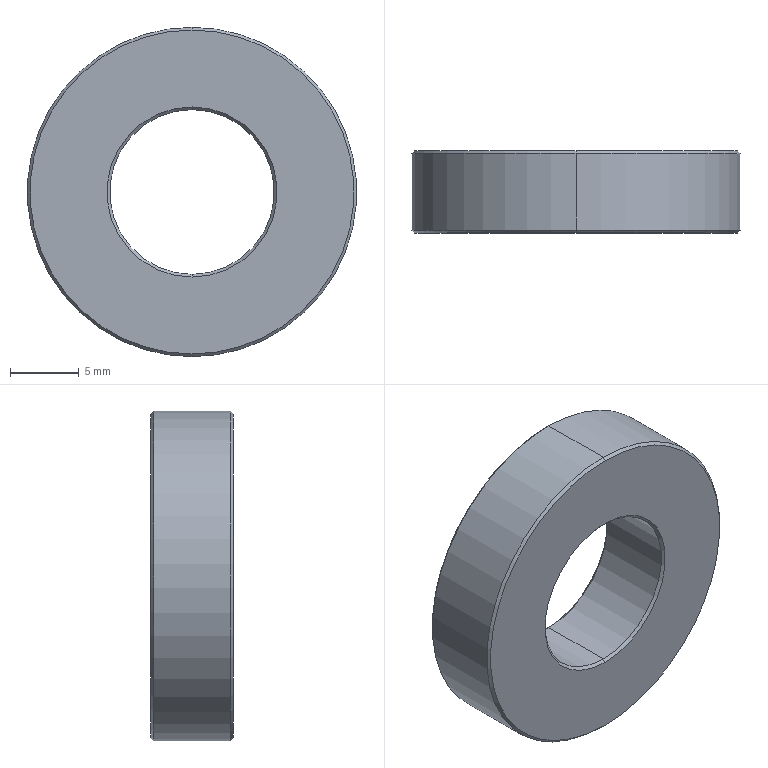Part | SolidWorks | features Chamfer 1, Extrusion 1 | 1 solid | 14 faces | box 24 x 6 x 24 mm | volume 2031 mm3 | cone 8 | cylinder 4 | plane 2 | commonest cylinder face diameters 12 x2 24 x2
STEP:
#1=CARTESIAN_POINT('',(0.,5.8,-6.));
#2=VERTEX_POINT('',#1);
#3=CARTESIAN_POINT('',(0.,5.8,6.));
#4=VERTEX_POINT('',#3);
#5=CARTESIAN_POINT('',(0.,5.8,0.));
#6=DIRECTION('',(0.,1.,0.));
#7=DIRECTION('',(0.,0.,1.));
#8=AXIS2_PLACEMENT_3D('',#5,#6,#7);
#9=CIRCLE('',#8,6.);
#10=EDGE_CURVE('',#2,#4,#9,.T.);
#11=ORIENTED_EDGE('',*,*,#10,.F.);
#12=CARTESIAN_POINT('',(0.,6.,-6.2));
#13=VERTEX_POINT('',#12);
#14=CARTESIAN_POINT('',(0.,5.8,-6.));
#15=DIRECTION('',(0.,0.7071,-0.7071));
#16=VECTOR('',#15,1000.);
#17=LINE('',#14,#16);
#18=EDGE_CURVE('',#2,#13,#17,.T.);
#19=ORIENTED_EDGE('',*,*,#18,.T.);
#20=CARTESIAN_POINT('',(0.,6.,6.2));
#21=VERTEX_POINT('',#20);
#22=CARTESIAN_POINT('',(0.,6.,0.));
#23=DIRECTION('',(0.,-1.,0.));
#24=DIRECTION('',(0.,0.,1.));
#25=AXIS2_PLACEMENT_3D('',#22,#23,#24);
#26=CIRCLE('',#25,6.2);
#27=EDGE_CURVE('',#21,#13,#26,.T.);
#28=ORIENTED_EDGE('',*,*,#27,.F.);
#29=CARTESIAN_POINT('',(0.,5.8,6.));
#30=DIRECTION('',(0.,0.7071,0.7071));
#31=VECTOR('',#30,1000.);
#32=LINE('',#29,#31);
#33=EDGE_CURVE('',#4,#21,#32,.T.);
#34=ORIENTED_EDGE('',*,*,#33,.F.);
#35=EDGE_LOOP('',(#11,#19,#28,#34));
#36=FACE_OUTER_BOUND('',#35,.T.);
#37=CARTESIAN_POINT('',(0.,5.8,0.));
#38=DIRECTION('',(0.,1.,0.));
#39=DIRECTION('',(0.,0.,1.));
#40=AXIS2_PLACEMENT_3D('',#37,#38,#39);
#41=CONICAL_SURFACE('',#40,6.,0.7854);
#42=ADVANCED_FACE('',(#36),#41,.F.);
#43=CARTESIAN_POINT('',(0.,6.,11.8));
#44=VERTEX_POINT('',#43);
#45=CARTESIAN_POINT('',(0.,6.,-11.8));
#46=VERTEX_POINT('',#45);
#47=CARTESIAN_POINT('',(0.,6.,0.));
#48=DIRECTION('',(0.,1.,0.));
#49=DIRECTION('',(0.,0.,1.));
#50=AXIS2_PLACEMENT_3D('',#47,#48,#49);
#51=CIRCLE('',#50,11.8);
#52=EDGE_CURVE('',#44,#46,#51,.T.);
#53=ORIENTED_EDGE('',*,*,#52,.F.);
#54=CARTESIAN_POINT('',(0.,5.8,12.));
#55=VERTEX_POINT('',#54);
#56=CARTESIAN_POINT('',(0.,6.,11.8));
#57=DIRECTION('',(0.,-0.7071,0.7071));
#58=VECTOR('',#57,1000.);
#59=LINE('',#56,#58);
#60=EDGE_CURVE('',#44,#55,#59,.T.);
#61=ORIENTED_EDGE('',*,*,#60,.T.);
#62=CARTESIAN_POINT('',(0.,5.8,-12.));
#63=VERTEX_POINT('',#62);
#64=CARTESIAN_POINT('',(0.,5.8,0.));
#65=DIRECTION('',(0.,-1.,0.));
#66=DIRECTION('',(0.,0.,1.));
#67=AXIS2_PLACEMENT_3D('',#64,#65,#66);
#68=CIRCLE('',#67,12.);
#69=EDGE_CURVE('',#63,#55,#68,.T.);
#70=ORIENTED_EDGE('',*,*,#69,.F.);
#71=CARTESIAN_POINT('',(0.,6.,-11.8));
#72=DIRECTION('',(0.,-0.7071,-0.7071));
#73=VECTOR('',#72,1000.);
#74=LINE('',#71,#73);
#75=EDGE_CURVE('',#46,#63,#74,.T.);
#76=ORIENTED_EDGE('',*,*,#75,.F.);
#77=EDGE_LOOP('',(#53,#61,#70,#76));
#78=FACE_OUTER_BOUND('',#77,.T.);
#79=CARTESIAN_POINT('',(0.,6.,0.));
#80=DIRECTION('',(0.,-1.,0.));
#81=DIRECTION('',(0.,0.,-1.));
#82=AXIS2_PLACEMENT_3D('',#79,#80,#81);
#83=CONICAL_SURFACE('',#82,11.8,0.7854);
#84=ADVANCED_FACE('',(#78),#83,.T.);
#85=CARTESIAN_POINT('',(0.,0.2,6.));
#86=VERTEX_POINT('',#85);
#87=CARTESIAN_POINT('',(0.,0.2,-6.));
#88=VERTEX_POINT('',#87);
#89=CARTESIAN_POINT('',(0.,0.2,0.));
#90=DIRECTION('',(0.,-1.,0.));
#91=DIRECTION('',(0.,0.,1.));
#92=AXIS2_PLACEMENT_3D('',#89,#90,#91);
#93=CIRCLE('',#92,6.);
#94=EDGE_CURVE('',#86,#88,#93,.T.);
#95=ORIENTED_EDGE('',*,*,#94,.F.);
#96=CARTESIAN_POINT('',(0.,0.,6.2));
#97=VERTEX_POINT('',#96);
#98=CARTESIAN_POINT('',(0.,0.,6.2));
#99=DIRECTION('',(0.,-0.7071,0.7071));
#100=VECTOR('',#99,1000.);
#101=LINE('',#98,#100);
#102=EDGE_CURVE('',#86,#97,#101,.T.);
#103=ORIENTED_EDGE('',*,*,#102,.T.);
#104=CARTESIAN_POINT('',(0.,0.,-6.2));
#105=VERTEX_POINT('',#104);
#106=CARTESIAN_POINT('',(0.,0.,0.));
#107=DIRECTION('',(0.,1.,0.));
#108=DIRECTION('',(0.,0.,1.));
#109=AXIS2_PLACEMENT_3D('',#106,#107,#108);
#110=CIRCLE('',#109,6.2);
#111=EDGE_CURVE('',#105,#97,#110,.T.);
#112=ORIENTED_EDGE('',*,*,#111,.F.);
#113=CARTESIAN_POINT('',(0.,0.,-6.2));
#114=DIRECTION('',(0.,-0.7071,-0.7071));
#115=VECTOR('',#114,1000.);
#116=LINE('',#113,#115);
#117=EDGE_CURVE('',#88,#105,#116,.T.);
#118=ORIENTED_EDGE('',*,*,#117,.F.);
#119=EDGE_LOOP('',(#95,#103,#112,#118));
#120=FACE_OUTER_BOUND('',#119,.T.);
#121=CARTESIAN_POINT('',(0.,0.,0.));
#122=DIRECTION('',(0.,-1.,0.));
#123=DIRECTION('',(0.,0.,-1.));
#124=AXIS2_PLACEMENT_3D('',#121,#122,#123);
#125=CONICAL_SURFACE('',#124,6.2,0.7854);
#126=ADVANCED_FACE('',(#120),#125,.F.);
#127=CARTESIAN_POINT('',(0.,0.,-11.8));
#128=VERTEX_POINT('',#127);
#129=CARTESIAN_POINT('',(0.,0.,11.8));
#130=VERTEX_POINT('',#129);
#131=CARTESIAN_POINT('',(0.,0.,0.));
#132=DIRECTION('',(0.,-1.,0.));
#133=DIRECTION('',(0.,0.,1.));
#134=AXIS2_PLACEMENT_3D('',#131,#132,#133);
#135=CIRCLE('',#134,11.8);
#136=EDGE_CURVE('',#128,#130,#135,.T.);
#137=ORIENTED_EDGE('',*,*,#136,.F.);
#138=CARTESIAN_POINT('',(0.,0.2,-12.));
#139=VERTEX_POINT('',#138);
#140=CARTESIAN_POINT('',(0.,0.2,-12.));
#141=DIRECTION('',(0.,0.7071,-0.7071));
#142=VECTOR('',#141,1000.);
#143=LINE('',#140,#142);
#144=EDGE_CURVE('',#128,#139,#143,.T.);
#145=ORIENTED_EDGE('',*,*,#144,.T.);
#146=CARTESIAN_POINT('',(0.,0.2,12.));
#147=VERTEX_POINT('',#146);
#148=CARTESIAN_POINT('',(0.,0.2,0.));
#149=DIRECTION('',(0.,1.,0.));
#150=DIRECTION('',(0.,0.,1.));
#151=AXIS2_PLACEMENT_3D('',#148,#149,#150);
#152=CIRCLE('',#151,12.);
#153=EDGE_CURVE('',#147,#139,#152,.T.);
#154=ORIENTED_EDGE('',*,*,#153,.F.);
#155=CARTESIAN_POINT('',(0.,0.2,12.));
#156=DIRECTION('',(0.,0.7071,0.7071));
#157=VECTOR('',#156,1000.);
#158=LINE('',#155,#157);
#159=EDGE_CURVE('',#130,#147,#158,.T.);
#160=ORIENTED_EDGE('',*,*,#159,.F.);
#161=EDGE_LOOP('',(#137,#145,#154,#160));
#162=FACE_OUTER_BOUND('',#161,.T.);
#163=CARTESIAN_POINT('',(0.,0.2,0.));
#164=DIRECTION('',(0.,1.,0.));
#165=DIRECTION('',(0.,0.,1.));
#166=AXIS2_PLACEMENT_3D('',#163,#164,#165);
#167=CONICAL_SURFACE('',#166,12.,0.7854);
#168=ADVANCED_FACE('',(#162),#167,.T.);
#169=ORIENTED_EDGE('',*,*,#10,.T.);
#170=CARTESIAN_POINT('',(0.,6.,6.));
#171=DIRECTION('',(0.,-1.,0.));
#172=VECTOR('',#171,1000.);
#173=LINE('',#170,#172);
#174=EDGE_CURVE('',#4,#86,#173,.T.);
#175=ORIENTED_EDGE('',*,*,#174,.T.);
#176=ORIENTED_EDGE('',*,*,#94,.T.);
#177=CARTESIAN_POINT('',(0.,6.,-6.));
#178=DIRECTION('',(0.,-1.,0.));
#179=VECTOR('',#178,1000.);
#180=LINE('',#177,#179);
#181=EDGE_CURVE('',#2,#88,#180,.T.);
#182=ORIENTED_EDGE('',*,*,#181,.F.);
#183=EDGE_LOOP('',(#169,#175,#176,#182));
#184=FACE_OUTER_BOUND('',#183,.T.);
#185=CARTESIAN_POINT('',(0.,6.,0.));
#186=DIRECTION('',(0.,-1.,0.));
#187=DIRECTION('',(0.,0.,-1.));
#188=AXIS2_PLACEMENT_3D('',#185,#186,#187);
#189=CYLINDRICAL_SURFACE('',#188,6.);
#190=ADVANCED_FACE('',(#184),#189,.F.);
#191=ORIENTED_EDGE('',*,*,#69,.T.);
#192=CARTESIAN_POINT('',(0.,6.,12.));
#193=DIRECTION('',(0.,-1.,0.));
#194=VECTOR('',#193,1000.);
#195=LINE('',#192,#194);
#196=EDGE_CURVE('',#55,#147,#195,.T.);
#197=ORIENTED_EDGE('',*,*,#196,.T.);
#198=ORIENTED_EDGE('',*,*,#153,.T.);
#199=CARTESIAN_POINT('',(0.,6.,-12.));
#200=DIRECTION('',(0.,-1.,0.));
#201=VECTOR('',#200,1000.);
#202=LINE('',#199,#201);
#203=EDGE_CURVE('',#63,#139,#202,.T.);
#204=ORIENTED_EDGE('',*,*,#203,.F.);
#205=EDGE_LOOP('',(#191,#197,#198,#204));
#206=FACE_OUTER_BOUND('',#205,.T.);
#207=CARTESIAN_POINT('',(0.,6.,0.));
#208=DIRECTION('',(0.,-1.,0.));
#209=DIRECTION('',(0.,0.,-1.));
#210=AXIS2_PLACEMENT_3D('',#207,#208,#209);
#211=CYLINDRICAL_SURFACE('',#210,12.);
#212=ADVANCED_FACE('',(#206),#211,.T.);
#213=CARTESIAN_POINT('',(0.,6.,0.));
#214=DIRECTION('',(0.,1.,0.));
#215=DIRECTION('',(0.,0.,1.));
#216=AXIS2_PLACEMENT_3D('',#213,#214,#215);
#217=CIRCLE('',#216,11.8);
#218=EDGE_CURVE('',#46,#44,#217,.T.);
#219=ORIENTED_EDGE('',*,*,#218,.T.);
#220=ORIENTED_EDGE('',*,*,#52,.T.);
#221=EDGE_LOOP('',(#219,#220));
#222=FACE_OUTER_BOUND('',#221,.T.);
#223=ORIENTED_EDGE('',*,*,#27,.T.);
#224=CARTESIAN_POINT('',(0.,6.,0.));
#225=DIRECTION('',(0.,-1.,0.));
#226=DIRECTION('',(0.,0.,1.));
#227=AXIS2_PLACEMENT_3D('',#224,#225,#226);
#228=CIRCLE('',#227,6.2);
#229=EDGE_CURVE('',#13,#21,#228,.T.);
#230=ORIENTED_EDGE('',*,*,#229,.T.);
#231=EDGE_LOOP('',(#223,#230));
#232=FACE_BOUND('',#231,.T.);
#233=CARTESIAN_POINT('',(0.,6.,0.));
#234=DIRECTION('',(0.,1.,0.));
#235=DIRECTION('',(0.,0.,1.));
#236=AXIS2_PLACEMENT_3D('',#233,#234,#235);
#237=PLANE('',#236);
#238=ADVANCED_FACE('',(#222,#232),#237,.T.);
#239=CARTESIAN_POINT('',(0.,0.,0.));
#240=DIRECTION('',(0.,-1.,0.));
#241=DIRECTION('',(0.,0.,1.));
#242=AXIS2_PLACEMENT_3D('',#239,#240,#241);
#243=CIRCLE('',#242,11.8);
#244=EDGE_CURVE('',#130,#128,#243,.T.);
#245=ORIENTED_EDGE('',*,*,#244,.T.);
#246=ORIENTED_EDGE('',*,*,#136,.T.);
#247=EDGE_LOOP('',(#245,#246));
#248=FACE_OUTER_BOUND('',#247,.T.);
#249=ORIENTED_EDGE('',*,*,#111,.T.);
#250=CARTESIAN_POINT('',(0.,0.,0.));
#251=DIRECTION('',(0.,1.,0.));
#252=DIRECTION('',(0.,0.,1.));
#253=AXIS2_PLACEMENT_3D('',#250,#251,#252);
#254=CIRCLE('',#253,6.2);
#255=EDGE_CURVE('',#97,#105,#254,.T.);
#256=ORIENTED_EDGE('',*,*,#255,.T.);
#257=EDGE_LOOP('',(#249,#256));
#258=FACE_BOUND('',#257,.T.);
#259=CARTESIAN_POINT('',(0.,0.,0.));
#260=DIRECTION('',(0.,1.,0.));
#261=DIRECTION('',(0.,0.,1.));
#262=AXIS2_PLACEMENT_3D('',#259,#260,#261);
#263=PLANE('',#262);
#264=ADVANCED_FACE('',(#248,#258),#263,.F.);
#265=ORIENTED_EDGE('',*,*,#196,.F.);
#266=CARTESIAN_POINT('',(0.,5.8,0.));
#267=DIRECTION('',(0.,-1.,0.));
#268=DIRECTION('',(0.,0.,1.));
#269=AXIS2_PLACEMENT_3D('',#266,#267,#268);
#270=CIRCLE('',#269,12.);
#271=EDGE_CURVE('',#55,#63,#270,.T.);
#272=ORIENTED_EDGE('',*,*,#271,.T.);
#273=ORIENTED_EDGE('',*,*,#203,.T.);
#274=CARTESIAN_POINT('',(0.,0.2,0.));
#275=DIRECTION('',(0.,1.,0.));
#276=DIRECTION('',(0.,0.,1.));
#277=AXIS2_PLACEMENT_3D('',#274,#275,#276);
#278=CIRCLE('',#277,12.);
#279=EDGE_CURVE('',#139,#147,#278,.T.);
#280=ORIENTED_EDGE('',*,*,#279,.T.);
#281=EDGE_LOOP('',(#265,#272,#273,#280));
#282=FACE_OUTER_BOUND('',#281,.T.);
#283=CARTESIAN_POINT('',(0.,6.,0.));
#284=DIRECTION('',(0.,-1.,0.));
#285=DIRECTION('',(0.,0.,-1.));
#286=AXIS2_PLACEMENT_3D('',#283,#284,#285);
#287=CYLINDRICAL_SURFACE('',#286,12.);
#288=ADVANCED_FACE('',(#282),#287,.T.);
#289=ORIENTED_EDGE('',*,*,#174,.F.);
#290=CARTESIAN_POINT('',(0.,5.8,0.));
#291=DIRECTION('',(0.,1.,0.));
#292=DIRECTION('',(0.,0.,1.));
#293=AXIS2_PLACEMENT_3D('',#290,#291,#292);
#294=CIRCLE('',#293,6.);
#295=EDGE_CURVE('',#4,#2,#294,.T.);
#296=ORIENTED_EDGE('',*,*,#295,.T.);
#297=ORIENTED_EDGE('',*,*,#181,.T.);
#298=CARTESIAN_POINT('',(0.,0.2,0.));
#299=DIRECTION('',(0.,-1.,0.));
#300=DIRECTION('',(0.,0.,1.));
#301=AXIS2_PLACEMENT_3D('',#298,#299,#300);
#302=CIRCLE('',#301,6.);
#303=EDGE_CURVE('',#88,#86,#302,.T.);
#304=ORIENTED_EDGE('',*,*,#303,.T.);
#305=EDGE_LOOP('',(#289,#296,#297,#304));
#306=FACE_OUTER_BOUND('',#305,.T.);
#307=CARTESIAN_POINT('',(0.,6.,0.));
#308=DIRECTION('',(0.,-1.,0.));
#309=DIRECTION('',(0.,0.,-1.));
#310=AXIS2_PLACEMENT_3D('',#307,#308,#309);
#311=CYLINDRICAL_SURFACE('',#310,6.);
#312=ADVANCED_FACE('',(#306),#311,.F.);
#313=ORIENTED_EDGE('',*,*,#144,.F.);
#314=ORIENTED_EDGE('',*,*,#244,.F.);
#315=ORIENTED_EDGE('',*,*,#159,.T.);
#316=ORIENTED_EDGE('',*,*,#279,.F.);
#317=EDGE_LOOP('',(#313,#314,#315,#316));
#318=FACE_OUTER_BOUND('',#317,.T.);
#319=CARTESIAN_POINT('',(0.,0.2,0.));
#320=DIRECTION('',(0.,1.,0.));
#321=DIRECTION('',(0.,0.,1.));
#322=AXIS2_PLACEMENT_3D('',#319,#320,#321);
#323=CONICAL_SURFACE('',#322,12.,0.7854);
#324=ADVANCED_FACE('',(#318),#323,.T.);
#325=ORIENTED_EDGE('',*,*,#102,.F.);
#326=ORIENTED_EDGE('',*,*,#303,.F.);
#327=ORIENTED_EDGE('',*,*,#117,.T.);
#328=ORIENTED_EDGE('',*,*,#255,.F.);
#329=EDGE_LOOP('',(#325,#326,#327,#328));
#330=FACE_OUTER_BOUND('',#329,.T.);
#331=CARTESIAN_POINT('',(0.,0.,0.));
#332=DIRECTION('',(0.,-1.,0.));
#333=DIRECTION('',(0.,0.,-1.));
#334=AXIS2_PLACEMENT_3D('',#331,#332,#333);
#335=CONICAL_SURFACE('',#334,6.2,0.7854);
#336=ADVANCED_FACE('',(#330),#335,.F.);
#337=ORIENTED_EDGE('',*,*,#60,.F.);
#338=ORIENTED_EDGE('',*,*,#218,.F.);
#339=ORIENTED_EDGE('',*,*,#75,.T.);
#340=ORIENTED_EDGE('',*,*,#271,.F.);
#341=EDGE_LOOP('',(#337,#338,#339,#340));
#342=FACE_OUTER_BOUND('',#341,.T.);
#343=CARTESIAN_POINT('',(0.,6.,0.));
#344=DIRECTION('',(0.,-1.,0.));
#345=DIRECTION('',(0.,0.,-1.));
#346=AXIS2_PLACEMENT_3D('',#343,#344,#345);
#347=CONICAL_SURFACE('',#346,11.8,0.7854);
#348=ADVANCED_FACE('',(#342),#347,.T.);
#349=ORIENTED_EDGE('',*,*,#18,.F.);
#350=ORIENTED_EDGE('',*,*,#295,.F.);
#351=ORIENTED_EDGE('',*,*,#33,.T.);
#352=ORIENTED_EDGE('',*,*,#229,.F.);
#353=EDGE_LOOP('',(#349,#350,#351,#352));
#354=FACE_OUTER_BOUND('',#353,.T.);
#355=CARTESIAN_POINT('',(0.,5.8,0.));
#356=DIRECTION('',(0.,1.,0.));
#357=DIRECTION('',(0.,0.,1.));
#358=AXIS2_PLACEMENT_3D('',#355,#356,#357);
#359=CONICAL_SURFACE('',#358,6.,0.7854);
#360=ADVANCED_FACE('',(#354),#359,.F.);
#361=CLOSED_SHELL('',(#42,#84,#126,#168,#190,#212,#238,#264,#288,#312,#324,#336,#348,#360));
#362=MANIFOLD_SOLID_BREP('',#361);
#363=CARTESIAN_POINT('',(0.,0.,0.));
#364=DIRECTION('',(0.,0.,1.));
#365=DIRECTION('',(1.,0.,0.));
#366=AXIS2_PLACEMENT_3D('',#363,#364,#365);
#367=(LENGTH_UNIT()NAMED_UNIT(*)SI_UNIT(.MILLI.,.METRE.));
#368=UNCERTAINTY_MEASURE_WITH_UNIT(LENGTH_MEASURE(0.00001),#367,'','');
#369=(NAMED_UNIT(*)PLANE_ANGLE_UNIT()SI_UNIT($,.RADIAN.));
#370=(NAMED_UNIT(*)SI_UNIT($,.STERADIAN.)SOLID_ANGLE_UNIT());
#371=(GEOMETRIC_REPRESENTATION_CONTEXT(3)GLOBAL_UNCERTAINTY_ASSIGNED_CONTEXT((#368))GLOBAL_UNIT_ASSIGNED_CONTEXT((#367,#369,#370))REPRESENTATION_CONTEXT('',''));
#372=ADVANCED_BREP_SHAPE_REPRESENTATION('',(#362,#366),#371);